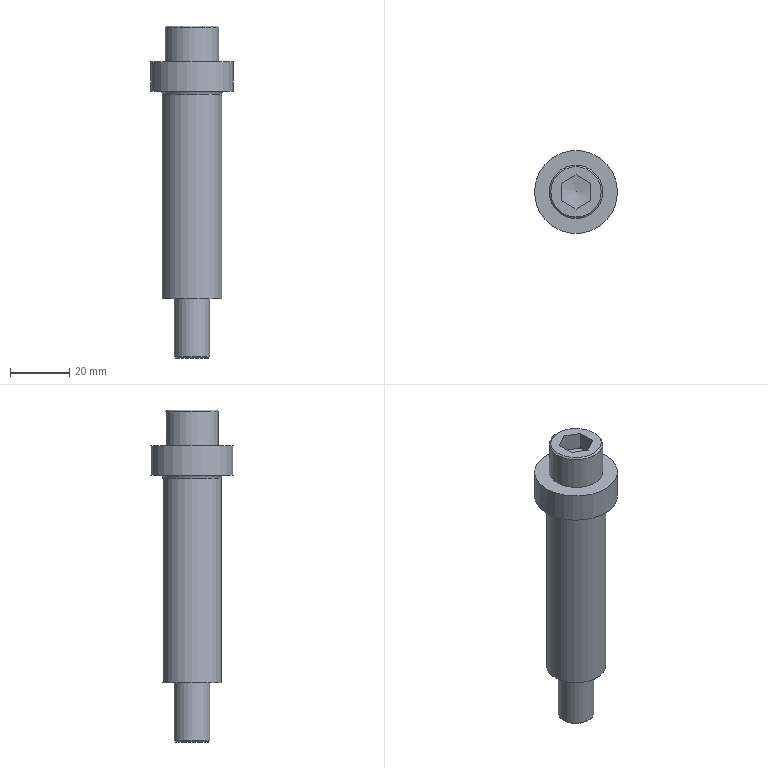Part | NX | features CSR20-100_1 2 | 1 solid | 27 faces | box 28 x 28 x 112 mm | volume 31985 mm3 | plane 18 | cylinder 5 | cone 3 | torus 1 | commonest cylinder face diameters 12 x1 12.6 x1 18 x1 20 x1 28 x1
STEP:
#1=CARTESIAN_POINT('',(1614.01,-26.667,109.999));
#2=VERTEX_POINT('',#1);
#3=CARTESIAN_POINT('',(1628.01,-26.667,109.999));
#4=DIRECTION('',(0.,0.,1.));
#5=DIRECTION('',(-1.,0.,0.));
#6=AXIS2_PLACEMENT_3D('',#3,#4,#5);
#7=CIRCLE('',#6,14.);
#8=EDGE_CURVE('',#2,#2,#7,.T.);
#9=ORIENTED_EDGE('',*,*,#8,.T.);
#10=EDGE_LOOP('',(#9));
#11=FACE_BOUND('',#10,.T.);
#12=CARTESIAN_POINT('',(1619.01,-26.667,109.999));
#13=VERTEX_POINT('',#12);
#14=CARTESIAN_POINT('',(1628.01,-26.667,109.999));
#15=DIRECTION('',(0.,0.,-1.));
#16=DIRECTION('',(-1.,0.,0.));
#17=AXIS2_PLACEMENT_3D('',#14,#15,#16);
#18=CIRCLE('',#17,9.);
#19=EDGE_CURVE('',#13,#13,#18,.T.);
#20=ORIENTED_EDGE('',*,*,#19,.T.);
#21=EDGE_LOOP('',(#20));
#22=FACE_BOUND('',#21,.T.);
#23=CARTESIAN_POINT('',(1628.01,-26.667,109.999));
#24=DIRECTION('',(0.,0.,1.));
#25=DIRECTION('',(-1.,0.,0.));
#26=AXIS2_PLACEMENT_3D('',#23,#24,#25);
#27=PLANE('',#26);
#28=ADVANCED_FACE('',(#11,#22),#27,.T.);
#29=CARTESIAN_POINT('',(1618.01,-26.667,29.999));
#30=VERTEX_POINT('',#29);
#31=CARTESIAN_POINT('',(1628.01,-26.667,29.999));
#32=DIRECTION('',(0.,0.,-1.));
#33=DIRECTION('',(-1.,0.,0.));
#34=AXIS2_PLACEMENT_3D('',#31,#32,#33);
#35=CIRCLE('',#34,10.);
#36=EDGE_CURVE('',#30,#30,#35,.T.);
#37=ORIENTED_EDGE('',*,*,#36,.F.);
#38=EDGE_LOOP('',(#37));
#39=FACE_BOUND('',#38,.T.);
#40=CARTESIAN_POINT('',(1618.01,-26.667,98.999));
#41=VERTEX_POINT('',#40);
#42=CARTESIAN_POINT('',(1628.01,-26.667,98.999));
#43=DIRECTION('',(0.,0.,1.));
#44=DIRECTION('',(1.,0.,0.));
#45=AXIS2_PLACEMENT_3D('',#42,#43,#44);
#46=CIRCLE('',#45,10.);
#47=EDGE_CURVE('',#41,#41,#46,.T.);
#48=ORIENTED_EDGE('',*,*,#47,.F.);
#49=EDGE_LOOP('',(#48));
#50=FACE_BOUND('',#49,.T.);
#51=CARTESIAN_POINT('',(1628.01,-26.667,79.999));
#52=DIRECTION('',(0.,0.,-1.));
#53=DIRECTION('',(1.,0.,0.));
#54=AXIS2_PLACEMENT_3D('',#51,#52,#53);
#55=CYLINDRICAL_SURFACE('',#54,10.);
#56=ADVANCED_FACE('',(#39,#50),#55,.T.);
#57=CARTESIAN_POINT('',(1621.71,-26.667,109.999));
#58=VERTEX_POINT('',#57);
#59=CARTESIAN_POINT('',(1628.01,-26.667,109.999));
#60=DIRECTION('',(0.,0.,-1.));
#61=DIRECTION('',(-1.,0.,0.));
#62=AXIS2_PLACEMENT_3D('',#59,#60,#61);
#63=CIRCLE('',#62,6.3);
#64=EDGE_CURVE('',#58,#58,#63,.T.);
#65=ORIENTED_EDGE('',*,*,#64,.F.);
#66=EDGE_LOOP('',(#65));
#67=FACE_BOUND('',#66,.T.);
#68=CARTESIAN_POINT('',(1621.71,-26.667,29.999));
#69=VERTEX_POINT('',#68);
#70=CARTESIAN_POINT('',(1628.01,-26.667,29.999));
#71=DIRECTION('',(0.,0.,1.));
#72=DIRECTION('',(-1.,0.,0.));
#73=AXIS2_PLACEMENT_3D('',#70,#71,#72);
#74=CIRCLE('',#73,6.3);
#75=EDGE_CURVE('',#69,#69,#74,.T.);
#76=ORIENTED_EDGE('',*,*,#75,.F.);
#77=EDGE_LOOP('',(#76));
#78=FACE_BOUND('',#77,.T.);
#79=CARTESIAN_POINT('',(1628.01,-26.667,84.999));
#80=DIRECTION('',(0.,0.,-1.));
#81=DIRECTION('',(1.,0.,0.));
#82=AXIS2_PLACEMENT_3D('',#79,#80,#81);
#83=CYLINDRICAL_SURFACE('',#82,6.3);
#84=ADVANCED_FACE('',(#67,#78),#83,.F.);
#85=ORIENTED_EDGE('',*,*,#47,.T.);
#86=EDGE_LOOP('',(#85));
#87=FACE_BOUND('',#86,.T.);
#88=CARTESIAN_POINT('',(1617.01,-26.667,99.999));
#89=VERTEX_POINT('',#88);
#90=CARTESIAN_POINT('',(1628.01,-26.667,99.999));
#91=DIRECTION('',(0.,0.,-1.));
#92=DIRECTION('',(1.,0.,0.));
#93=AXIS2_PLACEMENT_3D('',#90,#91,#92);
#94=CIRCLE('',#93,11.);
#95=EDGE_CURVE('',#89,#89,#94,.T.);
#96=ORIENTED_EDGE('',*,*,#95,.T.);
#97=EDGE_LOOP('',(#96));
#98=FACE_BOUND('',#97,.T.);
#99=CARTESIAN_POINT('',(1628.01,-26.667,98.999));
#100=DIRECTION('',(0.,0.,1.));
#101=DIRECTION('',(-1.,0.,0.));
#102=AXIS2_PLACEMENT_3D('',#99,#100,#101);
#103=TOROIDAL_SURFACE('',#102,11.,1.);
#104=ADVANCED_FACE('',(#87,#98),#103,.F.);
#105=CARTESIAN_POINT('',(1614.01,-26.667,99.999));
#106=VERTEX_POINT('',#105);
#107=CARTESIAN_POINT('',(1628.01,-26.667,99.999));
#108=DIRECTION('',(0.,0.,-1.));
#109=DIRECTION('',(-1.,0.,0.));
#110=AXIS2_PLACEMENT_3D('',#107,#108,#109);
#111=CIRCLE('',#110,14.);
#112=EDGE_CURVE('',#106,#106,#111,.T.);
#113=ORIENTED_EDGE('',*,*,#112,.T.);
#114=EDGE_LOOP('',(#113));
#115=FACE_BOUND('',#114,.T.);
#116=ORIENTED_EDGE('',*,*,#95,.F.);
#117=EDGE_LOOP('',(#116));
#118=FACE_BOUND('',#117,.T.);
#119=CARTESIAN_POINT('',(1628.01,-26.667,99.999));
#120=DIRECTION('',(0.,0.,-1.));
#121=DIRECTION('',(1.,0.,0.));
#122=AXIS2_PLACEMENT_3D('',#119,#120,#121);
#123=PLANE('',#122);
#124=ADVANCED_FACE('',(#115,#118),#123,.T.);
#125=ORIENTED_EDGE('',*,*,#75,.T.);
#126=EDGE_LOOP('',(#125));
#127=FACE_BOUND('',#126,.T.);
#128=ORIENTED_EDGE('',*,*,#36,.T.);
#129=EDGE_LOOP('',(#128));
#130=FACE_BOUND('',#129,.T.);
#131=CARTESIAN_POINT('',(1628.01,-26.667,29.999));
#132=DIRECTION('',(0.,0.,-1.));
#133=DIRECTION('',(1.,0.,0.));
#134=AXIS2_PLACEMENT_3D('',#131,#132,#133);
#135=PLANE('',#134);
#136=ADVANCED_FACE('',(#127,#130),#135,.T.);
#137=ORIENTED_EDGE('',*,*,#8,.F.);
#138=EDGE_LOOP('',(#137));
#139=FACE_BOUND('',#138,.T.);
#140=ORIENTED_EDGE('',*,*,#112,.F.);
#141=EDGE_LOOP('',(#140));
#142=FACE_BOUND('',#141,.T.);
#143=CARTESIAN_POINT('',(1628.01,-26.667,104.999));
#144=DIRECTION('',(0.,0.,-1.));
#145=DIRECTION('',(1.,0.,0.));
#146=AXIS2_PLACEMENT_3D('',#143,#144,#145);
#147=CYLINDRICAL_SURFACE('',#146,14.);
#148=ADVANCED_FACE('',(#139,#142),#147,.T.);
#149=CARTESIAN_POINT('',(1628.01,-32.441,121.999));
#150=VERTEX_POINT('',#149);
#151=CARTESIAN_POINT('',(1623.01,-29.554,121.999));
#152=VERTEX_POINT('',#151);
#153=CARTESIAN_POINT('',(1625.51,-30.997,121.999));
#154=DIRECTION('',(-0.866,0.5,0.));
#155=VECTOR('',#154,1000.);
#156=LINE('',#153,#155);
#157=EDGE_CURVE('',#150,#152,#156,.T.);
#158=ORIENTED_EDGE('',*,*,#157,.T.);
#159=CARTESIAN_POINT('',(1623.01,-23.78,121.999));
#160=VERTEX_POINT('',#159);
#161=CARTESIAN_POINT('',(1623.01,-26.667,121.999));
#162=DIRECTION('',(0.,1.,0.));
#163=VECTOR('',#162,1000.);
#164=LINE('',#161,#163);
#165=EDGE_CURVE('',#152,#160,#164,.T.);
#166=ORIENTED_EDGE('',*,*,#165,.T.);
#167=CARTESIAN_POINT('',(1628.01,-20.894,121.999));
#168=VERTEX_POINT('',#167);
#169=CARTESIAN_POINT('',(1625.51,-22.337,121.999));
#170=DIRECTION('',(0.866,0.5,0.));
#171=VECTOR('',#170,1000.);
#172=LINE('',#169,#171);
#173=EDGE_CURVE('',#160,#168,#172,.T.);
#174=ORIENTED_EDGE('',*,*,#173,.T.);
#175=CARTESIAN_POINT('',(1633.01,-23.78,121.999));
#176=VERTEX_POINT('',#175);
#177=CARTESIAN_POINT('',(1630.51,-22.337,121.999));
#178=DIRECTION('',(0.866,-0.5,0.));
#179=VECTOR('',#178,1000.);
#180=LINE('',#177,#179);
#181=EDGE_CURVE('',#168,#176,#180,.T.);
#182=ORIENTED_EDGE('',*,*,#181,.T.);
#183=CARTESIAN_POINT('',(1633.01,-29.554,121.999));
#184=VERTEX_POINT('',#183);
#185=CARTESIAN_POINT('',(1633.01,-26.667,121.999));
#186=DIRECTION('',(0.,-1.,0.));
#187=VECTOR('',#186,1000.);
#188=LINE('',#185,#187);
#189=EDGE_CURVE('',#176,#184,#188,.T.);
#190=ORIENTED_EDGE('',*,*,#189,.T.);
#191=CARTESIAN_POINT('',(1630.51,-30.997,121.999));
#192=DIRECTION('',(-0.866,-0.5,0.));
#193=VECTOR('',#192,1000.);
#194=LINE('',#191,#193);
#195=EDGE_CURVE('',#184,#150,#194,.T.);
#196=ORIENTED_EDGE('',*,*,#195,.T.);
#197=EDGE_LOOP('',(#158,#166,#174,#182,#190,#196));
#198=FACE_BOUND('',#197,.T.);
#199=CARTESIAN_POINT('',(1619.51,-26.667,121.999));
#200=VERTEX_POINT('',#199);
#201=CARTESIAN_POINT('',(1628.01,-26.667,121.999));
#202=DIRECTION('',(0.,0.,-1.));
#203=DIRECTION('',(1.,0.,0.));
#204=AXIS2_PLACEMENT_3D('',#201,#202,#203);
#205=CIRCLE('',#204,8.5);
#206=EDGE_CURVE('',#200,#200,#205,.T.);
#207=ORIENTED_EDGE('',*,*,#206,.F.);
#208=EDGE_LOOP('',(#207));
#209=FACE_BOUND('',#208,.T.);
#210=CARTESIAN_POINT('',(1628.01,-26.667,121.999));
#211=DIRECTION('',(0.,0.,1.));
#212=DIRECTION('',(-1.,0.,0.));
#213=AXIS2_PLACEMENT_3D('',#210,#211,#212);
#214=PLANE('',#213);
#215=ADVANCED_FACE('',(#198,#209),#214,.T.);
#216=ORIENTED_EDGE('',*,*,#19,.F.);
#217=EDGE_LOOP('',(#216));
#218=FACE_BOUND('',#217,.T.);
#219=CARTESIAN_POINT('',(1619.01,-26.667,121.499));
#220=VERTEX_POINT('',#219);
#221=CARTESIAN_POINT('',(1628.01,-26.667,121.499));
#222=DIRECTION('',(0.,0.,1.));
#223=DIRECTION('',(1.,0.,0.));
#224=AXIS2_PLACEMENT_3D('',#221,#222,#223);
#225=CIRCLE('',#224,9.);
#226=EDGE_CURVE('',#220,#220,#225,.T.);
#227=ORIENTED_EDGE('',*,*,#226,.F.);
#228=EDGE_LOOP('',(#227));
#229=FACE_BOUND('',#228,.T.);
#230=CARTESIAN_POINT('',(1628.01,-26.667,115.999));
#231=DIRECTION('',(0.,0.,-1.));
#232=DIRECTION('',(1.,0.,0.));
#233=AXIS2_PLACEMENT_3D('',#230,#231,#232);
#234=CYLINDRICAL_SURFACE('',#233,9.);
#235=ADVANCED_FACE('',(#218,#229),#234,.T.);
#236=ORIENTED_EDGE('',*,*,#226,.T.);
#237=EDGE_LOOP('',(#236));
#238=FACE_BOUND('',#237,.T.);
#239=ORIENTED_EDGE('',*,*,#206,.T.);
#240=EDGE_LOOP('',(#239));
#241=FACE_BOUND('',#240,.T.);
#242=CARTESIAN_POINT('',(1628.01,-26.667,121.999));
#243=DIRECTION('',(0.,0.,-1.));
#244=DIRECTION('',(-1.,0.,0.));
#245=AXIS2_PLACEMENT_3D('',#242,#243,#244);
#246=CONICAL_SURFACE('',#245,8.5,0.7854);
#247=ADVANCED_FACE('',(#238,#241),#246,.T.);
#248=CARTESIAN_POINT('',(1623.01,-29.554,115.999));
#249=VERTEX_POINT('',#248);
#250=CARTESIAN_POINT('',(1623.01,-29.554,118.999));
#251=DIRECTION('',(0.,0.,1.));
#252=VECTOR('',#251,1000.);
#253=LINE('',#250,#252);
#254=EDGE_CURVE('',#249,#152,#253,.T.);
#255=ORIENTED_EDGE('',*,*,#254,.F.);
#256=CARTESIAN_POINT('',(1623.01,-23.78,115.999));
#257=VERTEX_POINT('',#256);
#258=CARTESIAN_POINT('',(1623.01,-26.667,115.999));
#259=DIRECTION('',(0.,1.,0.));
#260=VECTOR('',#259,1000.);
#261=LINE('',#258,#260);
#262=EDGE_CURVE('',#249,#257,#261,.T.);
#263=ORIENTED_EDGE('',*,*,#262,.T.);
#264=CARTESIAN_POINT('',(1623.01,-23.78,118.999));
#265=DIRECTION('',(0.,0.,1.));
#266=VECTOR('',#265,1000.);
#267=LINE('',#264,#266);
#268=EDGE_CURVE('',#257,#160,#267,.T.);
#269=ORIENTED_EDGE('',*,*,#268,.T.);
#270=ORIENTED_EDGE('',*,*,#165,.F.);
#271=EDGE_LOOP('',(#255,#263,#269,#270));
#272=FACE_BOUND('',#271,.T.);
#273=CARTESIAN_POINT('',(1623.01,-26.667,118.999));
#274=DIRECTION('',(1.,0.,0.));
#275=DIRECTION('',(0.,0.,1.));
#276=AXIS2_PLACEMENT_3D('',#273,#274,#275);
#277=PLANE('',#276);
#278=ADVANCED_FACE('',(#272),#277,.T.);
#279=ORIENTED_EDGE('',*,*,#268,.F.);
#280=CARTESIAN_POINT('',(1628.01,-20.894,115.999));
#281=VERTEX_POINT('',#280);
#282=CARTESIAN_POINT('',(1625.51,-22.337,115.999));
#283=DIRECTION('',(0.866,0.5,0.));
#284=VECTOR('',#283,1000.);
#285=LINE('',#282,#284);
#286=EDGE_CURVE('',#257,#281,#285,.T.);
#287=ORIENTED_EDGE('',*,*,#286,.T.);
#288=CARTESIAN_POINT('',(1628.01,-20.894,118.999));
#289=DIRECTION('',(0.,0.,1.));
#290=VECTOR('',#289,1000.);
#291=LINE('',#288,#290);
#292=EDGE_CURVE('',#281,#168,#291,.T.);
#293=ORIENTED_EDGE('',*,*,#292,.T.);
#294=ORIENTED_EDGE('',*,*,#173,.F.);
#295=EDGE_LOOP('',(#279,#287,#293,#294));
#296=FACE_BOUND('',#295,.T.);
#297=CARTESIAN_POINT('',(1625.51,-22.337,118.999));
#298=DIRECTION('',(0.5,-0.866,0.));
#299=DIRECTION('',(0.,0.,1.));
#300=AXIS2_PLACEMENT_3D('',#297,#298,#299);
#301=PLANE('',#300);
#302=ADVANCED_FACE('',(#296),#301,.T.);
#303=ORIENTED_EDGE('',*,*,#292,.F.);
#304=CARTESIAN_POINT('',(1633.01,-23.78,115.999));
#305=VERTEX_POINT('',#304);
#306=CARTESIAN_POINT('',(1630.51,-22.337,115.999));
#307=DIRECTION('',(0.866,-0.5,0.));
#308=VECTOR('',#307,1000.);
#309=LINE('',#306,#308);
#310=EDGE_CURVE('',#281,#305,#309,.T.);
#311=ORIENTED_EDGE('',*,*,#310,.T.);
#312=CARTESIAN_POINT('',(1633.01,-23.78,118.999));
#313=DIRECTION('',(0.,0.,1.));
#314=VECTOR('',#313,1000.);
#315=LINE('',#312,#314);
#316=EDGE_CURVE('',#305,#176,#315,.T.);
#317=ORIENTED_EDGE('',*,*,#316,.T.);
#318=ORIENTED_EDGE('',*,*,#181,.F.);
#319=EDGE_LOOP('',(#303,#311,#317,#318));
#320=FACE_BOUND('',#319,.T.);
#321=CARTESIAN_POINT('',(1630.51,-22.337,118.999));
#322=DIRECTION('',(-0.5,-0.866,0.));
#323=DIRECTION('',(0.,0.,-1.));
#324=AXIS2_PLACEMENT_3D('',#321,#322,#323);
#325=PLANE('',#324);
#326=ADVANCED_FACE('',(#320),#325,.T.);
#327=ORIENTED_EDGE('',*,*,#316,.F.);
#328=CARTESIAN_POINT('',(1633.01,-29.554,115.999));
#329=VERTEX_POINT('',#328);
#330=CARTESIAN_POINT('',(1633.01,-26.667,115.999));
#331=DIRECTION('',(0.,-1.,0.));
#332=VECTOR('',#331,1000.);
#333=LINE('',#330,#332);
#334=EDGE_CURVE('',#305,#329,#333,.T.);
#335=ORIENTED_EDGE('',*,*,#334,.T.);
#336=CARTESIAN_POINT('',(1633.01,-29.554,118.999));
#337=DIRECTION('',(0.,0.,1.));
#338=VECTOR('',#337,1000.);
#339=LINE('',#336,#338);
#340=EDGE_CURVE('',#329,#184,#339,.T.);
#341=ORIENTED_EDGE('',*,*,#340,.T.);
#342=ORIENTED_EDGE('',*,*,#189,.F.);
#343=EDGE_LOOP('',(#327,#335,#341,#342));
#344=FACE_BOUND('',#343,.T.);
#345=CARTESIAN_POINT('',(1633.01,-26.667,118.999));
#346=DIRECTION('',(-1.,0.,0.));
#347=DIRECTION('',(0.,0.,-1.));
#348=AXIS2_PLACEMENT_3D('',#345,#346,#347);
#349=PLANE('',#348);
#350=ADVANCED_FACE('',(#344),#349,.T.);
#351=ORIENTED_EDGE('',*,*,#340,.F.);
#352=CARTESIAN_POINT('',(1628.01,-32.441,115.999));
#353=VERTEX_POINT('',#352);
#354=CARTESIAN_POINT('',(1630.51,-30.997,115.999));
#355=DIRECTION('',(-0.866,-0.5,0.));
#356=VECTOR('',#355,1000.);
#357=LINE('',#354,#356);
#358=EDGE_CURVE('',#329,#353,#357,.T.);
#359=ORIENTED_EDGE('',*,*,#358,.T.);
#360=CARTESIAN_POINT('',(1628.01,-32.441,118.999));
#361=DIRECTION('',(0.,0.,1.));
#362=VECTOR('',#361,1000.);
#363=LINE('',#360,#362);
#364=EDGE_CURVE('',#353,#150,#363,.T.);
#365=ORIENTED_EDGE('',*,*,#364,.T.);
#366=ORIENTED_EDGE('',*,*,#195,.F.);
#367=EDGE_LOOP('',(#351,#359,#365,#366));
#368=FACE_BOUND('',#367,.T.);
#369=CARTESIAN_POINT('',(1630.51,-30.997,118.999));
#370=DIRECTION('',(-0.5,0.866,0.));
#371=DIRECTION('',(0.,0.,-1.));
#372=AXIS2_PLACEMENT_3D('',#369,#370,#371);
#373=PLANE('',#372);
#374=ADVANCED_FACE('',(#368),#373,.T.);
#375=ORIENTED_EDGE('',*,*,#364,.F.);
#376=CARTESIAN_POINT('',(1625.51,-30.997,115.999));
#377=DIRECTION('',(-0.866,0.5,0.));
#378=VECTOR('',#377,1000.);
#379=LINE('',#376,#378);
#380=EDGE_CURVE('',#353,#249,#379,.T.);
#381=ORIENTED_EDGE('',*,*,#380,.T.);
#382=ORIENTED_EDGE('',*,*,#254,.T.);
#383=ORIENTED_EDGE('',*,*,#157,.F.);
#384=EDGE_LOOP('',(#375,#381,#382,#383));
#385=FACE_BOUND('',#384,.T.);
#386=CARTESIAN_POINT('',(1625.51,-30.997,118.999));
#387=DIRECTION('',(0.5,0.866,0.));
#388=DIRECTION('',(0.,0.,1.));
#389=AXIS2_PLACEMENT_3D('',#386,#387,#388);
#390=PLANE('',#389);
#391=ADVANCED_FACE('',(#385),#390,.T.);
#392=CARTESIAN_POINT('',(1628.01,-26.667,115.999));
#393=DIRECTION('',(0.,0.,1.));
#394=DIRECTION('',(-1.,0.,0.));
#395=AXIS2_PLACEMENT_3D('',#392,#393,#394);
#396=CIRCLE('',#395,5.774);
#397=EDGE_CURVE('',#257,#249,#396,.T.);
#398=ORIENTED_EDGE('',*,*,#397,.T.);
#399=CARTESIAN_POINT('',(1628.01,-26.667,115.999));
#400=DIRECTION('',(0.,0.,1.));
#401=DIRECTION('',(-1.,0.,0.));
#402=AXIS2_PLACEMENT_3D('',#399,#400,#401);
#403=CIRCLE('',#402,5.774);
#404=EDGE_CURVE('',#249,#353,#403,.T.);
#405=ORIENTED_EDGE('',*,*,#404,.T.);
#406=CARTESIAN_POINT('',(1628.01,-26.667,115.999));
#407=DIRECTION('',(0.,0.,1.));
#408=DIRECTION('',(-1.,0.,0.));
#409=AXIS2_PLACEMENT_3D('',#406,#407,#408);
#410=CIRCLE('',#409,5.774);
#411=EDGE_CURVE('',#353,#329,#410,.T.);
#412=ORIENTED_EDGE('',*,*,#411,.T.);
#413=CARTESIAN_POINT('',(1628.01,-26.667,115.999));
#414=DIRECTION('',(0.,0.,1.));
#415=DIRECTION('',(-1.,0.,0.));
#416=AXIS2_PLACEMENT_3D('',#413,#414,#415);
#417=CIRCLE('',#416,5.774);
#418=EDGE_CURVE('',#329,#305,#417,.T.);
#419=ORIENTED_EDGE('',*,*,#418,.T.);
#420=CARTESIAN_POINT('',(1628.01,-26.667,115.999));
#421=DIRECTION('',(0.,0.,1.));
#422=DIRECTION('',(-1.,0.,0.));
#423=AXIS2_PLACEMENT_3D('',#420,#421,#422);
#424=CIRCLE('',#423,5.774);
#425=EDGE_CURVE('',#305,#281,#424,.T.);
#426=ORIENTED_EDGE('',*,*,#425,.T.);
#427=CARTESIAN_POINT('',(1628.01,-26.667,115.999));
#428=DIRECTION('',(0.,0.,1.));
#429=DIRECTION('',(-1.,0.,0.));
#430=AXIS2_PLACEMENT_3D('',#427,#428,#429);
#431=CIRCLE('',#430,5.774);
#432=EDGE_CURVE('',#281,#257,#431,.T.);
#433=ORIENTED_EDGE('',*,*,#432,.T.);
#434=EDGE_LOOP('',(#398,#405,#412,#419,#426,#433));
#435=FACE_BOUND('',#434,.T.);
#436=CARTESIAN_POINT('',(1628.01,-26.667,114.999));
#437=VERTEX_POINT('',#436);
#438=VERTEX_LOOP('',#437);
#439=FACE_BOUND('',#438,.T.);
#440=CARTESIAN_POINT('',(1628.01,-26.667,115.499));
#441=DIRECTION('',(0.,0.,1.));
#442=DIRECTION('',(1.,0.,0.));
#443=AXIS2_PLACEMENT_3D('',#440,#441,#442);
#444=CONICAL_SURFACE('',#443,2.887,1.399);
#445=ADVANCED_FACE('',(#435,#439),#444,.F.);
#446=ORIENTED_EDGE('',*,*,#358,.F.);
#447=ORIENTED_EDGE('',*,*,#411,.F.);
#448=EDGE_LOOP('',(#446,#447));
#449=FACE_BOUND('',#448,.T.);
#450=CARTESIAN_POINT('',(1628.01,-26.667,115.999));
#451=DIRECTION('',(0.,0.,1.));
#452=DIRECTION('',(-1.,0.,0.));
#453=AXIS2_PLACEMENT_3D('',#450,#451,#452);
#454=PLANE('',#453);
#455=ADVANCED_FACE('',(#449),#454,.F.);
#456=ORIENTED_EDGE('',*,*,#334,.F.);
#457=ORIENTED_EDGE('',*,*,#418,.F.);
#458=EDGE_LOOP('',(#456,#457));
#459=FACE_BOUND('',#458,.T.);
#460=CARTESIAN_POINT('',(1628.01,-26.667,115.999));
#461=DIRECTION('',(0.,0.,1.));
#462=DIRECTION('',(-1.,0.,0.));
#463=AXIS2_PLACEMENT_3D('',#460,#461,#462);
#464=PLANE('',#463);
#465=ADVANCED_FACE('',(#459),#464,.F.);
#466=ORIENTED_EDGE('',*,*,#310,.F.);
#467=ORIENTED_EDGE('',*,*,#425,.F.);
#468=EDGE_LOOP('',(#466,#467));
#469=FACE_BOUND('',#468,.T.);
#470=CARTESIAN_POINT('',(1628.01,-26.667,115.999));
#471=DIRECTION('',(0.,0.,1.));
#472=DIRECTION('',(-1.,0.,0.));
#473=AXIS2_PLACEMENT_3D('',#470,#471,#472);
#474=PLANE('',#473);
#475=ADVANCED_FACE('',(#469),#474,.F.);
#476=ORIENTED_EDGE('',*,*,#286,.F.);
#477=ORIENTED_EDGE('',*,*,#432,.F.);
#478=EDGE_LOOP('',(#476,#477));
#479=FACE_BOUND('',#478,.T.);
#480=CARTESIAN_POINT('',(1628.01,-26.667,115.999));
#481=DIRECTION('',(0.,0.,1.));
#482=DIRECTION('',(-1.,0.,0.));
#483=AXIS2_PLACEMENT_3D('',#480,#481,#482);
#484=PLANE('',#483);
#485=ADVANCED_FACE('',(#479),#484,.F.);
#486=ORIENTED_EDGE('',*,*,#262,.F.);
#487=ORIENTED_EDGE('',*,*,#397,.F.);
#488=EDGE_LOOP('',(#486,#487));
#489=FACE_BOUND('',#488,.T.);
#490=CARTESIAN_POINT('',(1628.01,-26.667,115.999));
#491=DIRECTION('',(0.,0.,1.));
#492=DIRECTION('',(-1.,0.,0.));
#493=AXIS2_PLACEMENT_3D('',#490,#491,#492);
#494=PLANE('',#493);
#495=ADVANCED_FACE('',(#489),#494,.F.);
#496=ORIENTED_EDGE('',*,*,#380,.F.);
#497=ORIENTED_EDGE('',*,*,#404,.F.);
#498=EDGE_LOOP('',(#496,#497));
#499=FACE_BOUND('',#498,.T.);
#500=CARTESIAN_POINT('',(1628.01,-26.667,115.999));
#501=DIRECTION('',(0.,0.,1.));
#502=DIRECTION('',(-1.,0.,0.));
#503=AXIS2_PLACEMENT_3D('',#500,#501,#502);
#504=PLANE('',#503);
#505=ADVANCED_FACE('',(#499),#504,.F.);
#506=CARTESIAN_POINT('',(1622.01,-26.667,10.499));
#507=VERTEX_POINT('',#506);
#508=CARTESIAN_POINT('',(1628.01,-26.667,10.499));
#509=DIRECTION('',(0.,0.,-1.));
#510=DIRECTION('',(1.,0.,0.));
#511=AXIS2_PLACEMENT_3D('',#508,#509,#510);
#512=CIRCLE('',#511,6.);
#513=EDGE_CURVE('',#507,#507,#512,.T.);
#514=ORIENTED_EDGE('',*,*,#513,.T.);
#515=EDGE_LOOP('',(#514));
#516=FACE_BOUND('',#515,.T.);
#517=CARTESIAN_POINT('',(1622.51,-26.667,9.999));
#518=VERTEX_POINT('',#517);
#519=CARTESIAN_POINT('',(1628.01,-26.667,9.999));
#520=DIRECTION('',(0.,0.,1.));
#521=DIRECTION('',(1.,0.,0.));
#522=AXIS2_PLACEMENT_3D('',#519,#520,#521);
#523=CIRCLE('',#522,5.5);
#524=EDGE_CURVE('',#518,#518,#523,.T.);
#525=ORIENTED_EDGE('',*,*,#524,.T.);
#526=EDGE_LOOP('',(#525));
#527=FACE_BOUND('',#526,.T.);
#528=CARTESIAN_POINT('',(1628.01,-26.667,9.999));
#529=DIRECTION('',(0.,0.,1.));
#530=DIRECTION('',(-1.,0.,0.));
#531=AXIS2_PLACEMENT_3D('',#528,#529,#530);
#532=CONICAL_SURFACE('',#531,5.5,0.7854);
#533=ADVANCED_FACE('',(#516,#527),#532,.T.);
#534=CARTESIAN_POINT('',(1622.01,-26.667,109.999));
#535=VERTEX_POINT('',#534);
#536=CARTESIAN_POINT('',(1628.01,-26.667,109.999));
#537=DIRECTION('',(0.,0.,1.));
#538=DIRECTION('',(-1.,0.,0.));
#539=AXIS2_PLACEMENT_3D('',#536,#537,#538);
#540=CIRCLE('',#539,6.);
#541=EDGE_CURVE('',#535,#535,#540,.T.);
#542=ORIENTED_EDGE('',*,*,#541,.F.);
#543=EDGE_LOOP('',(#542));
#544=FACE_BOUND('',#543,.T.);
#545=ORIENTED_EDGE('',*,*,#513,.F.);
#546=EDGE_LOOP('',(#545));
#547=FACE_BOUND('',#546,.T.);
#548=CARTESIAN_POINT('',(1628.01,-26.667,74.999));
#549=DIRECTION('',(0.,0.,-1.));
#550=DIRECTION('',(1.,0.,0.));
#551=AXIS2_PLACEMENT_3D('',#548,#549,#550);
#552=CYLINDRICAL_SURFACE('',#551,6.);
#553=ADVANCED_FACE('',(#544,#547),#552,.T.);
#554=ORIENTED_EDGE('',*,*,#524,.F.);
#555=EDGE_LOOP('',(#554));
#556=FACE_BOUND('',#555,.T.);
#557=CARTESIAN_POINT('',(1628.01,-26.667,9.999));
#558=DIRECTION('',(0.,0.,-1.));
#559=DIRECTION('',(1.,0.,0.));
#560=AXIS2_PLACEMENT_3D('',#557,#558,#559);
#561=PLANE('',#560);
#562=ADVANCED_FACE('',(#556),#561,.T.);
#563=ORIENTED_EDGE('',*,*,#64,.T.);
#564=EDGE_LOOP('',(#563));
#565=FACE_BOUND('',#564,.T.);
#566=ORIENTED_EDGE('',*,*,#541,.T.);
#567=EDGE_LOOP('',(#566));
#568=FACE_BOUND('',#567,.T.);
#569=CARTESIAN_POINT('',(1628.01,-26.667,109.999));
#570=DIRECTION('',(0.,0.,-1.));
#571=DIRECTION('',(1.,0.,0.));
#572=AXIS2_PLACEMENT_3D('',#569,#570,#571);
#573=PLANE('',#572);
#574=ADVANCED_FACE('',(#565,#568),#573,.T.);
#575=CLOSED_SHELL('',(#28,#56,#84,#104,#124,#136,#148,#215,#235,#247,#278,#302,#326,#350,#374,#391,#445,#455,#465,#475,#485,#495,#505,#533,#553,#562,#574));
#576=MANIFOLD_SOLID_BREP('',#575);
#577=(LENGTH_UNIT()NAMED_UNIT(*)SI_UNIT(.MILLI.,.METRE.));
#578=UNCERTAINTY_MEASURE_WITH_UNIT(LENGTH_MEASURE(0.00001),#577,'','');
#579=(NAMED_UNIT(*)PLANE_ANGLE_UNIT()SI_UNIT($,.RADIAN.));
#580=(NAMED_UNIT(*)SI_UNIT($,.STERADIAN.)SOLID_ANGLE_UNIT());
#581=(GEOMETRIC_REPRESENTATION_CONTEXT(3)GLOBAL_UNCERTAINTY_ASSIGNED_CONTEXT((#578))GLOBAL_UNIT_ASSIGNED_CONTEXT((#577,#579,#580))REPRESENTATION_CONTEXT('',''));
#582=ADVANCED_BREP_SHAPE_REPRESENTATION('',(#576),#581);